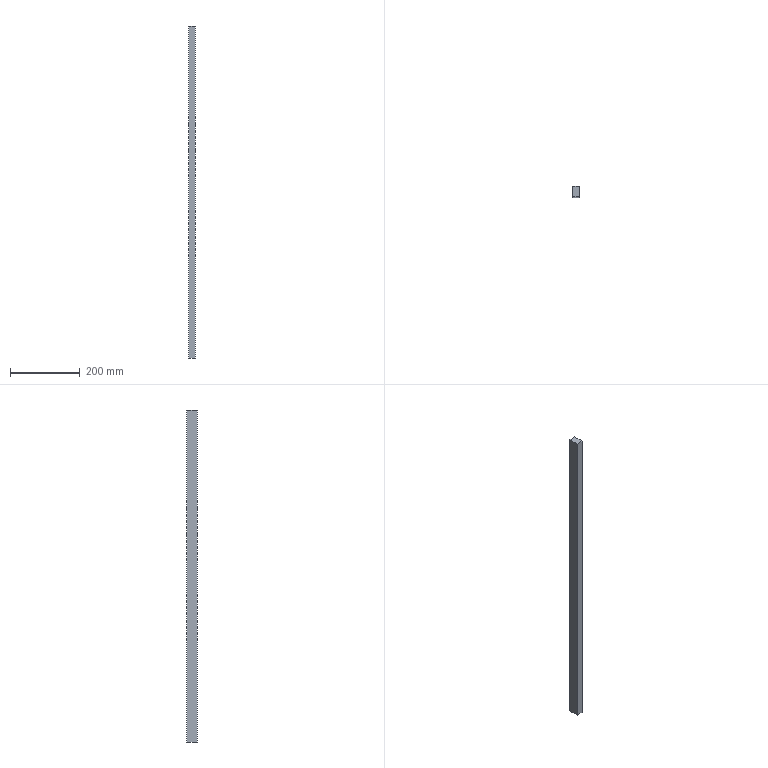Part | STEP file | Grating | 1 solid | 6 faces | box 20 x 30 x 950 mm | volume 570000 mm3 | plane 6
STEP:
#1=CARTESIAN_POINT('',(0.,0.,0.));
#2=DIRECTION('',(0.,0.,1.));
#3=DIRECTION('',(1.,0.,0.));
#4=AXIS2_PLACEMENT_3D('',#1,#2,#3);
#5=CARTESIAN_POINT('',(0.,0.,0.));
#6=VERTEX_POINT('',#5);
#7=CARTESIAN_POINT('',(0.,-30.,0.));
#8=VERTEX_POINT('',#7);
#9=CARTESIAN_POINT('',(0.,0.,0.));
#10=DIRECTION('',(0.,-1.,0.));
#11=VECTOR('',#10,1.);
#12=LINE('',#9,#11);
#13=CARTESIAN_POINT('',(20.,0.,0.));
#14=DIRECTION('',(0.,0.,-1.));
#15=DIRECTION('',(0.,1.,0.));
#16=AXIS2_PLACEMENT_3D('',#13,#14,#15);
#17=PLANE('',#16);
#18=CARTESIAN_POINT('',(0.,-20.));
#19=DIRECTION('',(-1.,0.));
#20=VECTOR('',#19,1.);
#21=LINE('',#18,#20);
#22=(GEOMETRIC_REPRESENTATION_CONTEXT(2)PARAMETRIC_REPRESENTATION_CONTEXT()REPRESENTATION_CONTEXT('',''));
#23=DEFINITIONAL_REPRESENTATION('',(#21),#22);
#24=PCURVE('',#17,#23);
#25=CARTESIAN_POINT('',(0.,0.,0.));
#26=DIRECTION('',(1.,0.,0.));
#27=DIRECTION('',(0.,0.,-1.));
#28=AXIS2_PLACEMENT_3D('',#25,#26,#27);
#29=PLANE('',#28);
#30=CARTESIAN_POINT('',(0.,0.));
#31=DIRECTION('',(0.,-1.));
#32=VECTOR('',#31,1.);
#33=LINE('',#30,#32);
#34=(GEOMETRIC_REPRESENTATION_CONTEXT(2)PARAMETRIC_REPRESENTATION_CONTEXT()REPRESENTATION_CONTEXT('',''));
#35=DEFINITIONAL_REPRESENTATION('',(#33),#34);
#36=PCURVE('',#29,#35);
#37=SURFACE_CURVE('',#12,(#24,#36),.PCURVE_S1.);
#38=EDGE_CURVE('',#6,#8,#37,.T.);
#39=ORIENTED_EDGE('',*,*,#38,.T.);
#40=CARTESIAN_POINT('',(20.,-30.,0.));
#41=VERTEX_POINT('',#40);
#42=CARTESIAN_POINT('',(20.,-30.,0.));
#43=DIRECTION('',(-1.,0.,0.));
#44=VECTOR('',#43,1.);
#45=LINE('',#42,#44);
#46=CARTESIAN_POINT('',(-30.,0.));
#47=DIRECTION('',(0.,-1.));
#48=VECTOR('',#47,1.);
#49=LINE('',#46,#48);
#50=(GEOMETRIC_REPRESENTATION_CONTEXT(2)PARAMETRIC_REPRESENTATION_CONTEXT()REPRESENTATION_CONTEXT('',''));
#51=DEFINITIONAL_REPRESENTATION('',(#49),#50);
#52=PCURVE('',#17,#51);
#53=CARTESIAN_POINT('',(20.,-30.,0.));
#54=DIRECTION('',(0.,1.,0.));
#55=DIRECTION('',(0.,0.,1.));
#56=AXIS2_PLACEMENT_3D('',#53,#54,#55);
#57=PLANE('',#56);
#58=CARTESIAN_POINT('',(0.,0.));
#59=DIRECTION('',(0.,-1.));
#60=VECTOR('',#59,1.);
#61=LINE('',#58,#60);
#62=(GEOMETRIC_REPRESENTATION_CONTEXT(2)PARAMETRIC_REPRESENTATION_CONTEXT()REPRESENTATION_CONTEXT('',''));
#63=DEFINITIONAL_REPRESENTATION('',(#61),#62);
#64=PCURVE('',#57,#63);
#65=SURFACE_CURVE('',#45,(#52,#64),.PCURVE_S1.);
#66=EDGE_CURVE('',#41,#8,#65,.T.);
#67=ORIENTED_EDGE('',*,*,#66,.F.);
#68=CARTESIAN_POINT('',(20.,0.,0.));
#69=VERTEX_POINT('',#68);
#70=CARTESIAN_POINT('',(20.,0.,0.));
#71=DIRECTION('',(0.,-1.,0.));
#72=VECTOR('',#71,1.);
#73=LINE('',#70,#72);
#74=CARTESIAN_POINT('',(0.,0.));
#75=DIRECTION('',(-1.,0.));
#76=VECTOR('',#75,1.);
#77=LINE('',#74,#76);
#78=(GEOMETRIC_REPRESENTATION_CONTEXT(2)PARAMETRIC_REPRESENTATION_CONTEXT()REPRESENTATION_CONTEXT('',''));
#79=DEFINITIONAL_REPRESENTATION('',(#77),#78);
#80=PCURVE('',#17,#79);
#81=CARTESIAN_POINT('',(20.,0.,0.));
#82=DIRECTION('',(1.,0.,0.));
#83=DIRECTION('',(0.,0.,-1.));
#84=AXIS2_PLACEMENT_3D('',#81,#82,#83);
#85=PLANE('',#84);
#86=CARTESIAN_POINT('',(0.,0.));
#87=DIRECTION('',(0.,-1.));
#88=VECTOR('',#87,1.);
#89=LINE('',#86,#88);
#90=(GEOMETRIC_REPRESENTATION_CONTEXT(2)PARAMETRIC_REPRESENTATION_CONTEXT()REPRESENTATION_CONTEXT('',''));
#91=DEFINITIONAL_REPRESENTATION('',(#89),#90);
#92=PCURVE('',#85,#91);
#93=SURFACE_CURVE('',#73,(#80,#92),.PCURVE_S1.);
#94=EDGE_CURVE('',#69,#41,#93,.T.);
#95=ORIENTED_EDGE('',*,*,#94,.F.);
#96=CARTESIAN_POINT('',(20.,0.,0.));
#97=DIRECTION('',(-1.,0.,0.));
#98=VECTOR('',#97,1.);
#99=LINE('',#96,#98);
#100=CARTESIAN_POINT('',(0.,0.));
#101=DIRECTION('',(0.,-1.));
#102=VECTOR('',#101,1.);
#103=LINE('',#100,#102);
#104=(GEOMETRIC_REPRESENTATION_CONTEXT(2)PARAMETRIC_REPRESENTATION_CONTEXT()REPRESENTATION_CONTEXT('',''));
#105=DEFINITIONAL_REPRESENTATION('',(#103),#104);
#106=PCURVE('',#17,#105);
#107=CARTESIAN_POINT('',(20.,0.,0.));
#108=DIRECTION('',(0.,-1.,0.));
#109=DIRECTION('',(0.,0.,-1.));
#110=AXIS2_PLACEMENT_3D('',#107,#108,#109);
#111=PLANE('',#110);
#112=CARTESIAN_POINT('',(0.,0.));
#113=DIRECTION('',(0.,-1.));
#114=VECTOR('',#113,1.);
#115=LINE('',#112,#114);
#116=(GEOMETRIC_REPRESENTATION_CONTEXT(2)PARAMETRIC_REPRESENTATION_CONTEXT()REPRESENTATION_CONTEXT('',''));
#117=DEFINITIONAL_REPRESENTATION('',(#115),#116);
#118=PCURVE('',#111,#117);
#119=SURFACE_CURVE('',#99,(#106,#118),.PCURVE_S1.);
#120=EDGE_CURVE('',#69,#6,#119,.T.);
#121=ORIENTED_EDGE('',*,*,#120,.T.);
#122=EDGE_LOOP('',(#39,#67,#95,#121));
#123=FACE_BOUND('',#122,.T.);
#124=ADVANCED_FACE('',(#123),#17,.F.);
#125=CARTESIAN_POINT('',(0.,-30.,-950.));
#126=VERTEX_POINT('',#125);
#127=CARTESIAN_POINT('',(0.,-30.,0.));
#128=DIRECTION('',(0.,0.,-1.));
#129=VECTOR('',#128,1.);
#130=LINE('',#127,#129);
#131=CARTESIAN_POINT('',(0.,-20.));
#132=DIRECTION('',(-1.,0.));
#133=VECTOR('',#132,1.);
#134=LINE('',#131,#133);
#135=(GEOMETRIC_REPRESENTATION_CONTEXT(2)PARAMETRIC_REPRESENTATION_CONTEXT()REPRESENTATION_CONTEXT('',''));
#136=DEFINITIONAL_REPRESENTATION('',(#134),#135);
#137=PCURVE('',#57,#136);
#138=CARTESIAN_POINT('',(0.,-30.));
#139=DIRECTION('',(1.,0.));
#140=VECTOR('',#139,1.);
#141=LINE('',#138,#140);
#142=(GEOMETRIC_REPRESENTATION_CONTEXT(2)PARAMETRIC_REPRESENTATION_CONTEXT()REPRESENTATION_CONTEXT('',''));
#143=DEFINITIONAL_REPRESENTATION('',(#141),#142);
#144=PCURVE('',#29,#143);
#145=SURFACE_CURVE('',#130,(#137,#144),.PCURVE_S1.);
#146=EDGE_CURVE('',#8,#126,#145,.T.);
#147=ORIENTED_EDGE('',*,*,#146,.T.);
#148=CARTESIAN_POINT('',(20.,-30.,-950.));
#149=VERTEX_POINT('',#148);
#150=CARTESIAN_POINT('',(20.,-30.,-950.));
#151=DIRECTION('',(-1.,0.,0.));
#152=VECTOR('',#151,1.);
#153=LINE('',#150,#152);
#154=CARTESIAN_POINT('',(-950.,0.));
#155=DIRECTION('',(0.,-1.));
#156=VECTOR('',#155,1.);
#157=LINE('',#154,#156);
#158=(GEOMETRIC_REPRESENTATION_CONTEXT(2)PARAMETRIC_REPRESENTATION_CONTEXT()REPRESENTATION_CONTEXT('',''));
#159=DEFINITIONAL_REPRESENTATION('',(#157),#158);
#160=PCURVE('',#57,#159);
#161=CARTESIAN_POINT('',(20.,0.,-950.));
#162=DIRECTION('',(0.,0.,1.));
#163=DIRECTION('',(1.,0.,0.));
#164=AXIS2_PLACEMENT_3D('',#161,#162,#163);
#165=PLANE('',#164);
#166=CARTESIAN_POINT('',(0.,-30.));
#167=DIRECTION('',(-1.,0.));
#168=VECTOR('',#167,1.);
#169=LINE('',#166,#168);
#170=(GEOMETRIC_REPRESENTATION_CONTEXT(2)PARAMETRIC_REPRESENTATION_CONTEXT()REPRESENTATION_CONTEXT('',''));
#171=DEFINITIONAL_REPRESENTATION('',(#169),#170);
#172=PCURVE('',#165,#171);
#173=SURFACE_CURVE('',#153,(#160,#172),.PCURVE_S1.);
#174=EDGE_CURVE('',#149,#126,#173,.T.);
#175=ORIENTED_EDGE('',*,*,#174,.F.);
#176=CARTESIAN_POINT('',(20.,-30.,0.));
#177=DIRECTION('',(0.,0.,-1.));
#178=VECTOR('',#177,1.);
#179=LINE('',#176,#178);
#180=CARTESIAN_POINT('',(0.,0.));
#181=DIRECTION('',(-1.,0.));
#182=VECTOR('',#181,1.);
#183=LINE('',#180,#182);
#184=(GEOMETRIC_REPRESENTATION_CONTEXT(2)PARAMETRIC_REPRESENTATION_CONTEXT()REPRESENTATION_CONTEXT('',''));
#185=DEFINITIONAL_REPRESENTATION('',(#183),#184);
#186=PCURVE('',#57,#185);
#187=CARTESIAN_POINT('',(0.,-30.));
#188=DIRECTION('',(1.,0.));
#189=VECTOR('',#188,1.);
#190=LINE('',#187,#189);
#191=(GEOMETRIC_REPRESENTATION_CONTEXT(2)PARAMETRIC_REPRESENTATION_CONTEXT()REPRESENTATION_CONTEXT('',''));
#192=DEFINITIONAL_REPRESENTATION('',(#190),#191);
#193=PCURVE('',#85,#192);
#194=SURFACE_CURVE('',#179,(#186,#193),.PCURVE_S1.);
#195=EDGE_CURVE('',#41,#149,#194,.T.);
#196=ORIENTED_EDGE('',*,*,#195,.F.);
#197=ORIENTED_EDGE('',*,*,#66,.T.);
#198=EDGE_LOOP('',(#147,#175,#196,#197));
#199=FACE_BOUND('',#198,.T.);
#200=ADVANCED_FACE('',(#199),#57,.F.);
#201=CARTESIAN_POINT('',(0.,0.,-950.));
#202=VERTEX_POINT('',#201);
#203=CARTESIAN_POINT('',(0.,0.,-950.));
#204=DIRECTION('',(0.,1.,0.));
#205=VECTOR('',#204,1.);
#206=LINE('',#203,#205);
#207=CARTESIAN_POINT('',(-20.,0.));
#208=DIRECTION('',(0.,1.));
#209=VECTOR('',#208,1.);
#210=LINE('',#207,#209);
#211=(GEOMETRIC_REPRESENTATION_CONTEXT(2)PARAMETRIC_REPRESENTATION_CONTEXT()REPRESENTATION_CONTEXT('',''));
#212=DEFINITIONAL_REPRESENTATION('',(#210),#211);
#213=PCURVE('',#165,#212);
#214=CARTESIAN_POINT('',(950.,0.));
#215=DIRECTION('',(0.,1.));
#216=VECTOR('',#215,1.);
#217=LINE('',#214,#216);
#218=(GEOMETRIC_REPRESENTATION_CONTEXT(2)PARAMETRIC_REPRESENTATION_CONTEXT()REPRESENTATION_CONTEXT('',''));
#219=DEFINITIONAL_REPRESENTATION('',(#217),#218);
#220=PCURVE('',#29,#219);
#221=SURFACE_CURVE('',#206,(#213,#220),.PCURVE_S1.);
#222=EDGE_CURVE('',#126,#202,#221,.T.);
#223=ORIENTED_EDGE('',*,*,#222,.T.);
#224=CARTESIAN_POINT('',(20.,0.,-950.));
#225=VERTEX_POINT('',#224);
#226=CARTESIAN_POINT('',(20.,0.,-950.));
#227=DIRECTION('',(-1.,0.,0.));
#228=VECTOR('',#227,1.);
#229=LINE('',#226,#228);
#230=CARTESIAN_POINT('',(0.,0.));
#231=DIRECTION('',(-1.,0.));
#232=VECTOR('',#231,1.);
#233=LINE('',#230,#232);
#234=(GEOMETRIC_REPRESENTATION_CONTEXT(2)PARAMETRIC_REPRESENTATION_CONTEXT()REPRESENTATION_CONTEXT('',''));
#235=DEFINITIONAL_REPRESENTATION('',(#233),#234);
#236=PCURVE('',#165,#235);
#237=CARTESIAN_POINT('',(950.,0.));
#238=DIRECTION('',(0.,-1.));
#239=VECTOR('',#238,1.);
#240=LINE('',#237,#239);
#241=(GEOMETRIC_REPRESENTATION_CONTEXT(2)PARAMETRIC_REPRESENTATION_CONTEXT()REPRESENTATION_CONTEXT('',''));
#242=DEFINITIONAL_REPRESENTATION('',(#240),#241);
#243=PCURVE('',#111,#242);
#244=SURFACE_CURVE('',#229,(#236,#243),.PCURVE_S1.);
#245=EDGE_CURVE('',#225,#202,#244,.T.);
#246=ORIENTED_EDGE('',*,*,#245,.F.);
#247=CARTESIAN_POINT('',(20.,0.,-950.));
#248=DIRECTION('',(0.,1.,0.));
#249=VECTOR('',#248,1.);
#250=LINE('',#247,#249);
#251=CARTESIAN_POINT('',(0.,0.));
#252=DIRECTION('',(0.,1.));
#253=VECTOR('',#252,1.);
#254=LINE('',#251,#253);
#255=(GEOMETRIC_REPRESENTATION_CONTEXT(2)PARAMETRIC_REPRESENTATION_CONTEXT()REPRESENTATION_CONTEXT('',''));
#256=DEFINITIONAL_REPRESENTATION('',(#254),#255);
#257=PCURVE('',#165,#256);
#258=CARTESIAN_POINT('',(950.,0.));
#259=DIRECTION('',(0.,1.));
#260=VECTOR('',#259,1.);
#261=LINE('',#258,#260);
#262=(GEOMETRIC_REPRESENTATION_CONTEXT(2)PARAMETRIC_REPRESENTATION_CONTEXT()REPRESENTATION_CONTEXT('',''));
#263=DEFINITIONAL_REPRESENTATION('',(#261),#262);
#264=PCURVE('',#85,#263);
#265=SURFACE_CURVE('',#250,(#257,#264),.PCURVE_S1.);
#266=EDGE_CURVE('',#149,#225,#265,.T.);
#267=ORIENTED_EDGE('',*,*,#266,.F.);
#268=ORIENTED_EDGE('',*,*,#174,.T.);
#269=EDGE_LOOP('',(#223,#246,#267,#268));
#270=FACE_BOUND('',#269,.T.);
#271=ADVANCED_FACE('',(#270),#165,.F.);
#272=CARTESIAN_POINT('',(0.,0.,0.));
#273=DIRECTION('',(0.,0.,1.));
#274=VECTOR('',#273,1.);
#275=LINE('',#272,#274);
#276=CARTESIAN_POINT('',(0.,-20.));
#277=DIRECTION('',(-1.,0.));
#278=VECTOR('',#277,1.);
#279=LINE('',#276,#278);
#280=(GEOMETRIC_REPRESENTATION_CONTEXT(2)PARAMETRIC_REPRESENTATION_CONTEXT()REPRESENTATION_CONTEXT('',''));
#281=DEFINITIONAL_REPRESENTATION('',(#279),#280);
#282=PCURVE('',#111,#281);
#283=CARTESIAN_POINT('',(0.,0.));
#284=DIRECTION('',(-1.,0.));
#285=VECTOR('',#284,1.);
#286=LINE('',#283,#285);
#287=(GEOMETRIC_REPRESENTATION_CONTEXT(2)PARAMETRIC_REPRESENTATION_CONTEXT()REPRESENTATION_CONTEXT('',''));
#288=DEFINITIONAL_REPRESENTATION('',(#286),#287);
#289=PCURVE('',#29,#288);
#290=SURFACE_CURVE('',#275,(#282,#289),.PCURVE_S1.);
#291=EDGE_CURVE('',#202,#6,#290,.T.);
#292=ORIENTED_EDGE('',*,*,#291,.T.);
#293=ORIENTED_EDGE('',*,*,#120,.F.);
#294=CARTESIAN_POINT('',(20.,0.,0.));
#295=DIRECTION('',(0.,0.,1.));
#296=VECTOR('',#295,1.);
#297=LINE('',#294,#296);
#298=CARTESIAN_POINT('',(0.,0.));
#299=DIRECTION('',(-1.,0.));
#300=VECTOR('',#299,1.);
#301=LINE('',#298,#300);
#302=(GEOMETRIC_REPRESENTATION_CONTEXT(2)PARAMETRIC_REPRESENTATION_CONTEXT()REPRESENTATION_CONTEXT('',''));
#303=DEFINITIONAL_REPRESENTATION('',(#301),#302);
#304=PCURVE('',#111,#303);
#305=CARTESIAN_POINT('',(0.,0.));
#306=DIRECTION('',(-1.,0.));
#307=VECTOR('',#306,1.);
#308=LINE('',#305,#307);
#309=(GEOMETRIC_REPRESENTATION_CONTEXT(2)PARAMETRIC_REPRESENTATION_CONTEXT()REPRESENTATION_CONTEXT('',''));
#310=DEFINITIONAL_REPRESENTATION('',(#308),#309);
#311=PCURVE('',#85,#310);
#312=SURFACE_CURVE('',#297,(#304,#311),.PCURVE_S1.);
#313=EDGE_CURVE('',#225,#69,#312,.T.);
#314=ORIENTED_EDGE('',*,*,#313,.F.);
#315=ORIENTED_EDGE('',*,*,#245,.T.);
#316=EDGE_LOOP('',(#292,#293,#314,#315));
#317=FACE_BOUND('',#316,.T.);
#318=ADVANCED_FACE('',(#317),#111,.F.);
#319=ORIENTED_EDGE('',*,*,#94,.T.);
#320=ORIENTED_EDGE('',*,*,#195,.T.);
#321=ORIENTED_EDGE('',*,*,#266,.T.);
#322=ORIENTED_EDGE('',*,*,#313,.T.);
#323=EDGE_LOOP('',(#319,#320,#321,#322));
#324=FACE_BOUND('',#323,.T.);
#325=ADVANCED_FACE('',(#324),#85,.T.);
#326=ORIENTED_EDGE('',*,*,#38,.F.);
#327=ORIENTED_EDGE('',*,*,#291,.F.);
#328=ORIENTED_EDGE('',*,*,#222,.F.);
#329=ORIENTED_EDGE('',*,*,#146,.F.);
#330=EDGE_LOOP('',(#326,#327,#328,#329));
#331=FACE_BOUND('',#330,.T.);
#332=ADVANCED_FACE('',(#331),#29,.F.);
#333=CLOSED_SHELL('',(#124,#200,#271,#318,#325,#332));
#334=MANIFOLD_SOLID_BREP('',#333);
#335=(LENGTH_UNIT()NAMED_UNIT(*)SI_UNIT(.MILLI.,.METRE.));
#336=UNCERTAINTY_MEASURE_WITH_UNIT(LENGTH_MEASURE(0.0000001),#335,'','');
#337=(NAMED_UNIT(*)PLANE_ANGLE_UNIT()SI_UNIT($,.RADIAN.));
#338=(NAMED_UNIT(*)SI_UNIT($,.STERADIAN.)SOLID_ANGLE_UNIT());
#339=(GEOMETRIC_REPRESENTATION_CONTEXT(3)GLOBAL_UNCERTAINTY_ASSIGNED_CONTEXT((#336))GLOBAL_UNIT_ASSIGNED_CONTEXT((#335,#337,#338))REPRESENTATION_CONTEXT('',''));
#340=ADVANCED_BREP_SHAPE_REPRESENTATION('',(#4,#334),#339);